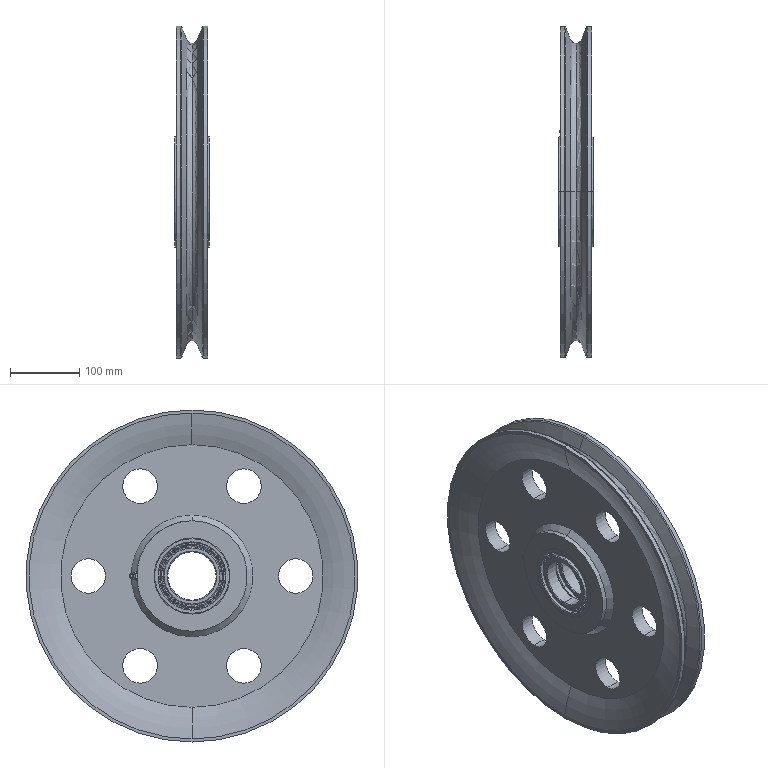Part | SolidWorks | features CompositeCurve 1 | 52 solids | 645 faces | box 50 x 480 x 480 mm | volume 4092545 mm3 | cylinder 248 | sphere 192 | plane 129 | torus 56 | cone 20 | commonest cylinder face diameters 88 x90 92 x90 50 x12 83.333 x8 96.667 x8 110 x8